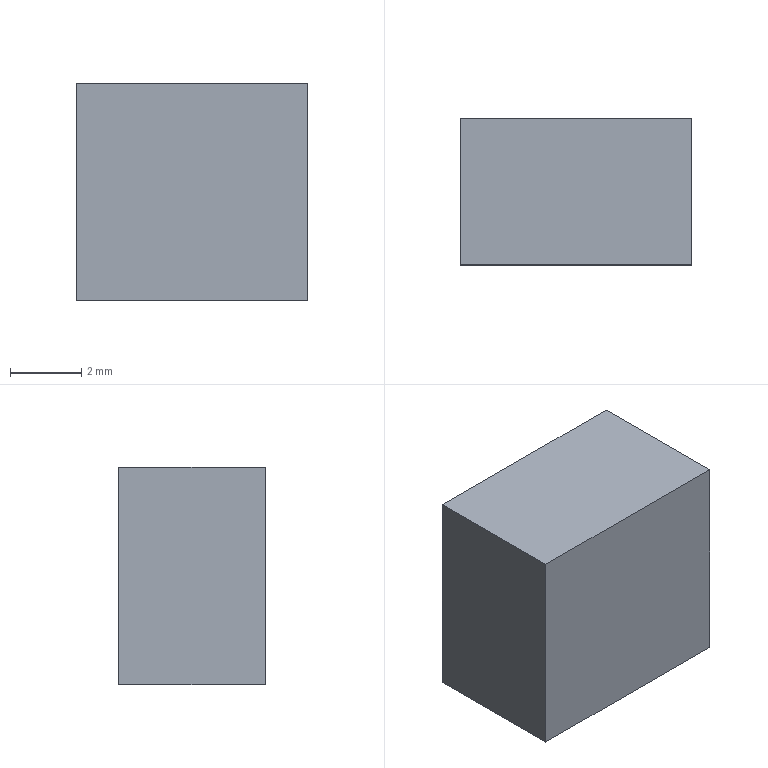Part | SolidWorks | features Extrusion 1 | 1 solid | 6 faces | box 6.5 x 4.1 x 6.1 mm | volume 162.565 mm3 | plane 6
STEP:
#1=CARTESIAN_POINT('',(0.,0.,-6.1));
#2=VERTEX_POINT('',#1);
#3=CARTESIAN_POINT('',(0.,0.,0.));
#4=VERTEX_POINT('',#3);
#5=CARTESIAN_POINT('',(0.,0.,0.));
#6=DIRECTION('',(0.,0.,1.));
#7=VECTOR('',#6,1000.);
#8=LINE('',#5,#7);
#9=EDGE_CURVE('',#2,#4,#8,.T.);
#10=ORIENTED_EDGE('',*,*,#9,.T.);
#11=CARTESIAN_POINT('',(0.,4.1,0.));
#12=VERTEX_POINT('',#11);
#13=CARTESIAN_POINT('',(0.,4.1,0.));
#14=DIRECTION('',(0.,-1.,0.));
#15=VECTOR('',#14,1000.);
#16=LINE('',#13,#15);
#17=EDGE_CURVE('',#12,#4,#16,.T.);
#18=ORIENTED_EDGE('',*,*,#17,.F.);
#19=CARTESIAN_POINT('',(0.,4.1,-6.1));
#20=VERTEX_POINT('',#19);
#21=CARTESIAN_POINT('',(0.,4.1,0.));
#22=DIRECTION('',(0.,0.,1.));
#23=VECTOR('',#22,1000.);
#24=LINE('',#21,#23);
#25=EDGE_CURVE('',#20,#12,#24,.T.);
#26=ORIENTED_EDGE('',*,*,#25,.F.);
#27=CARTESIAN_POINT('',(0.,4.1,-6.1));
#28=DIRECTION('',(0.,-1.,0.));
#29=VECTOR('',#28,1000.);
#30=LINE('',#27,#29);
#31=EDGE_CURVE('',#20,#2,#30,.T.);
#32=ORIENTED_EDGE('',*,*,#31,.T.);
#33=EDGE_LOOP('',(#10,#18,#26,#32));
#34=FACE_OUTER_BOUND('',#33,.T.);
#35=CARTESIAN_POINT('',(0.,4.1,0.));
#36=DIRECTION('',(1.,0.,0.));
#37=DIRECTION('',(0.,0.,-1.));
#38=AXIS2_PLACEMENT_3D('',#35,#36,#37);
#39=PLANE('',#38);
#40=ADVANCED_FACE('',(#34),#39,.F.);
#41=CARTESIAN_POINT('',(6.5,0.,0.));
#42=VERTEX_POINT('',#41);
#43=CARTESIAN_POINT('',(0.,0.,0.));
#44=DIRECTION('',(1.,0.,0.));
#45=VECTOR('',#44,1000.);
#46=LINE('',#43,#45);
#47=EDGE_CURVE('',#4,#42,#46,.T.);
#48=ORIENTED_EDGE('',*,*,#47,.T.);
#49=CARTESIAN_POINT('',(6.5,4.1,0.));
#50=VERTEX_POINT('',#49);
#51=CARTESIAN_POINT('',(6.5,4.1,0.));
#52=DIRECTION('',(0.,-1.,0.));
#53=VECTOR('',#52,1000.);
#54=LINE('',#51,#53);
#55=EDGE_CURVE('',#50,#42,#54,.T.);
#56=ORIENTED_EDGE('',*,*,#55,.F.);
#57=CARTESIAN_POINT('',(0.,4.1,0.));
#58=DIRECTION('',(1.,0.,0.));
#59=VECTOR('',#58,1000.);
#60=LINE('',#57,#59);
#61=EDGE_CURVE('',#12,#50,#60,.T.);
#62=ORIENTED_EDGE('',*,*,#61,.F.);
#63=ORIENTED_EDGE('',*,*,#17,.T.);
#64=EDGE_LOOP('',(#48,#56,#62,#63));
#65=FACE_OUTER_BOUND('',#64,.T.);
#66=CARTESIAN_POINT('',(0.,4.1,0.));
#67=DIRECTION('',(0.,0.,-1.));
#68=DIRECTION('',(-1.,0.,0.));
#69=AXIS2_PLACEMENT_3D('',#66,#67,#68);
#70=PLANE('',#69);
#71=ADVANCED_FACE('',(#65),#70,.F.);
#72=CARTESIAN_POINT('',(6.5,0.,-6.1));
#73=VERTEX_POINT('',#72);
#74=CARTESIAN_POINT('',(6.5,0.,0.));
#75=DIRECTION('',(0.,0.,-1.));
#76=VECTOR('',#75,1000.);
#77=LINE('',#74,#76);
#78=EDGE_CURVE('',#42,#73,#77,.T.);
#79=ORIENTED_EDGE('',*,*,#78,.T.);
#80=CARTESIAN_POINT('',(6.5,4.1,-6.1));
#81=VERTEX_POINT('',#80);
#82=CARTESIAN_POINT('',(6.5,4.1,-6.1));
#83=DIRECTION('',(0.,-1.,0.));
#84=VECTOR('',#83,1000.);
#85=LINE('',#82,#84);
#86=EDGE_CURVE('',#81,#73,#85,.T.);
#87=ORIENTED_EDGE('',*,*,#86,.F.);
#88=CARTESIAN_POINT('',(6.5,4.1,0.));
#89=DIRECTION('',(0.,0.,-1.));
#90=VECTOR('',#89,1000.);
#91=LINE('',#88,#90);
#92=EDGE_CURVE('',#50,#81,#91,.T.);
#93=ORIENTED_EDGE('',*,*,#92,.F.);
#94=ORIENTED_EDGE('',*,*,#55,.T.);
#95=EDGE_LOOP('',(#79,#87,#93,#94));
#96=FACE_OUTER_BOUND('',#95,.T.);
#97=CARTESIAN_POINT('',(6.5,4.1,0.));
#98=DIRECTION('',(-1.,0.,0.));
#99=DIRECTION('',(0.,0.,1.));
#100=AXIS2_PLACEMENT_3D('',#97,#98,#99);
#101=PLANE('',#100);
#102=ADVANCED_FACE('',(#96),#101,.F.);
#103=CARTESIAN_POINT('',(0.,0.,-6.1));
#104=DIRECTION('',(-1.,0.,0.));
#105=VECTOR('',#104,1000.);
#106=LINE('',#103,#105);
#107=EDGE_CURVE('',#73,#2,#106,.T.);
#108=ORIENTED_EDGE('',*,*,#107,.T.);
#109=ORIENTED_EDGE('',*,*,#31,.F.);
#110=CARTESIAN_POINT('',(0.,4.1,-6.1));
#111=DIRECTION('',(-1.,0.,0.));
#112=VECTOR('',#111,1000.);
#113=LINE('',#110,#112);
#114=EDGE_CURVE('',#81,#20,#113,.T.);
#115=ORIENTED_EDGE('',*,*,#114,.F.);
#116=ORIENTED_EDGE('',*,*,#86,.T.);
#117=EDGE_LOOP('',(#108,#109,#115,#116));
#118=FACE_OUTER_BOUND('',#117,.T.);
#119=CARTESIAN_POINT('',(0.,4.1,-6.1));
#120=DIRECTION('',(0.,0.,1.));
#121=DIRECTION('',(1.,0.,0.));
#122=AXIS2_PLACEMENT_3D('',#119,#120,#121);
#123=PLANE('',#122);
#124=ADVANCED_FACE('',(#118),#123,.F.);
#125=ORIENTED_EDGE('',*,*,#25,.T.);
#126=ORIENTED_EDGE('',*,*,#61,.T.);
#127=ORIENTED_EDGE('',*,*,#92,.T.);
#128=ORIENTED_EDGE('',*,*,#114,.T.);
#129=EDGE_LOOP('',(#125,#126,#127,#128));
#130=FACE_OUTER_BOUND('',#129,.T.);
#131=CARTESIAN_POINT('',(0.,4.1,0.));
#132=DIRECTION('',(0.,-1.,0.));
#133=DIRECTION('',(0.,0.,-1.));
#134=AXIS2_PLACEMENT_3D('',#131,#132,#133);
#135=PLANE('',#134);
#136=ADVANCED_FACE('',(#130),#135,.F.);
#137=ORIENTED_EDGE('',*,*,#9,.F.);
#138=ORIENTED_EDGE('',*,*,#107,.F.);
#139=ORIENTED_EDGE('',*,*,#78,.F.);
#140=ORIENTED_EDGE('',*,*,#47,.F.);
#141=EDGE_LOOP('',(#137,#138,#139,#140));
#142=FACE_OUTER_BOUND('',#141,.T.);
#143=CARTESIAN_POINT('',(0.,0.,0.));
#144=DIRECTION('',(0.,-1.,0.));
#145=DIRECTION('',(0.,0.,-1.));
#146=AXIS2_PLACEMENT_3D('',#143,#144,#145);
#147=PLANE('',#146);
#148=ADVANCED_FACE('',(#142),#147,.T.);
#149=CLOSED_SHELL('',(#40,#71,#102,#124,#136,#148));
#150=MANIFOLD_SOLID_BREP('',#149);
#151=CARTESIAN_POINT('',(0.,0.,0.));
#152=DIRECTION('',(0.,0.,1.));
#153=DIRECTION('',(1.,0.,0.));
#154=AXIS2_PLACEMENT_3D('',#151,#152,#153);
#155=(LENGTH_UNIT()NAMED_UNIT(*)SI_UNIT(.MILLI.,.METRE.));
#156=UNCERTAINTY_MEASURE_WITH_UNIT(LENGTH_MEASURE(0.00001),#155,'','');
#157=(NAMED_UNIT(*)PLANE_ANGLE_UNIT()SI_UNIT($,.RADIAN.));
#158=(NAMED_UNIT(*)SI_UNIT($,.STERADIAN.)SOLID_ANGLE_UNIT());
#159=(GEOMETRIC_REPRESENTATION_CONTEXT(3)GLOBAL_UNCERTAINTY_ASSIGNED_CONTEXT((#156))GLOBAL_UNIT_ASSIGNED_CONTEXT((#155,#157,#158))REPRESENTATION_CONTEXT('',''));
#160=ADVANCED_BREP_SHAPE_REPRESENTATION('',(#150,#154),#159);